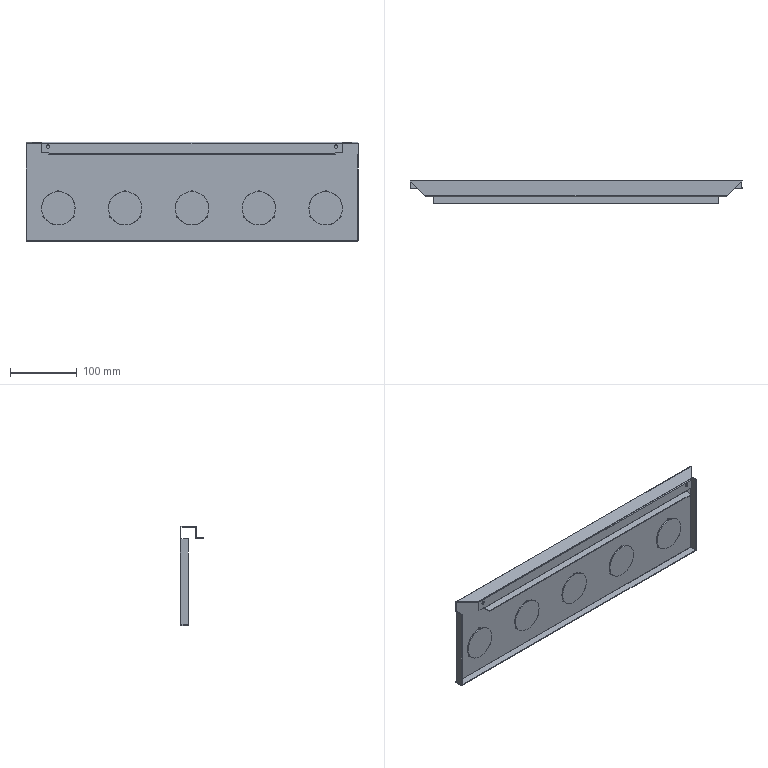Part | SolidWorks | features EdgeFlange 6, FlatPattern 1, FormToolInstance 1, ICE 1, LPattern 1, SMBaseFlange 1, SheetMetal 1 | 1 solid | 299 faces | box 497 x 35.8 x 148.8 mm | volume 125691 mm3 | plane 156 | cylinder 111 | spline 32 | commonest cylinder face diameters 50 x35 0.4 x21 2.8 x21 0.8 x15 3.2 x15 5.2 x4